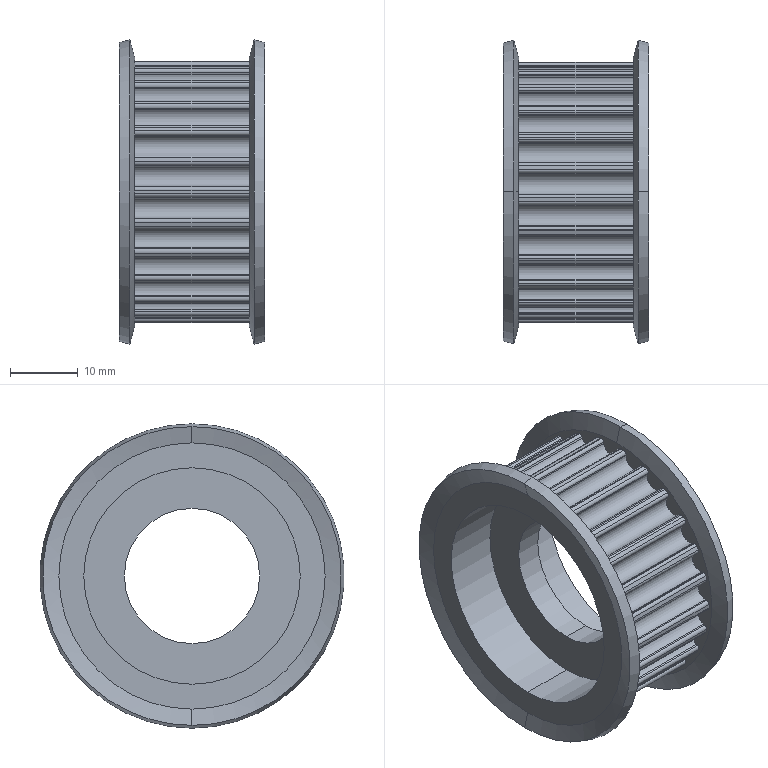Part | STEP file | C-HTPA25H5M150-A-N14 push-film driven pulley SGN-3-05 | 1 solid | 199 faces | box 21.487 x 45 x 45 mm | volume 8237 mm3 | cylinder 131 | plane 56 | cone 12 | commonest cylinder face diameters 1 x63 3.12 x37 38.65 x25 32 x4 20 x2